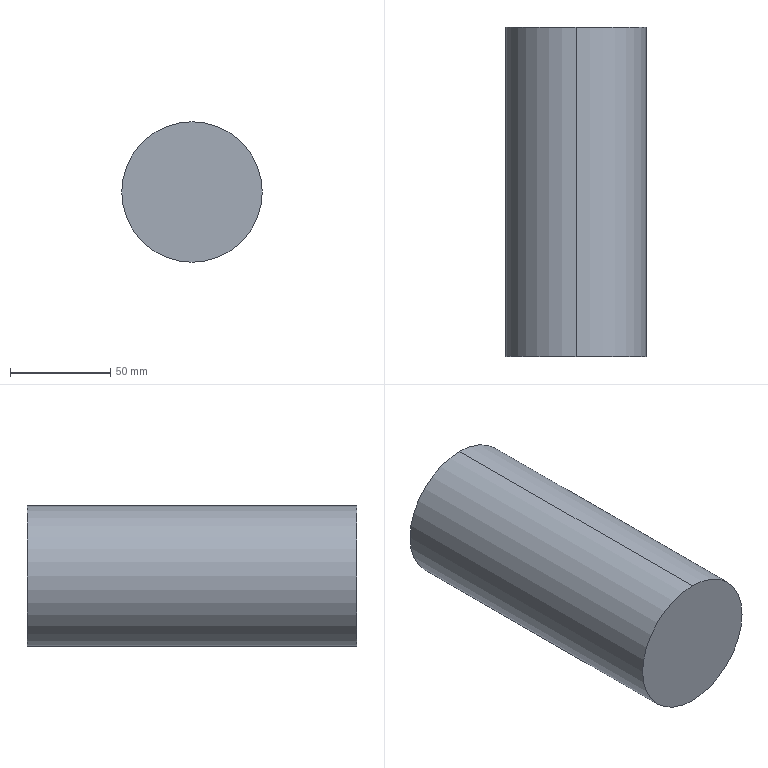Part | SolidWorks | features Extrusion 1 | 1 solid | 4 faces | box 70 x 163.9 x 70 mm | volume 630761 mm3 | cylinder 2 | plane 2 | commonest cylinder face diameters 70 x2
STEP:
#1=CARTESIAN_POINT('',(0.,163.9,35.));
#2=VERTEX_POINT('',#1);
#3=CARTESIAN_POINT('',(0.,163.9,-35.));
#4=VERTEX_POINT('',#3);
#5=CARTESIAN_POINT('',(0.,163.9,0.));
#6=DIRECTION('',(0.,1.,0.));
#7=DIRECTION('',(0.,0.,1.));
#8=AXIS2_PLACEMENT_3D('',#5,#6,#7);
#9=CIRCLE('',#8,35.);
#10=EDGE_CURVE('',#2,#4,#9,.T.);
#11=ORIENTED_EDGE('',*,*,#10,.F.);
#12=CARTESIAN_POINT('',(0.,0.,35.));
#13=VERTEX_POINT('',#12);
#14=CARTESIAN_POINT('',(0.,163.9,35.));
#15=DIRECTION('',(0.,-1.,0.));
#16=VECTOR('',#15,1000.);
#17=LINE('',#14,#16);
#18=EDGE_CURVE('',#2,#13,#17,.T.);
#19=ORIENTED_EDGE('',*,*,#18,.T.);
#20=CARTESIAN_POINT('',(0.,0.,-35.));
#21=VERTEX_POINT('',#20);
#22=CARTESIAN_POINT('',(0.,0.,0.));
#23=DIRECTION('',(0.,1.,0.));
#24=DIRECTION('',(0.,0.,1.));
#25=AXIS2_PLACEMENT_3D('',#22,#23,#24);
#26=CIRCLE('',#25,35.);
#27=EDGE_CURVE('',#13,#21,#26,.T.);
#28=ORIENTED_EDGE('',*,*,#27,.T.);
#29=CARTESIAN_POINT('',(0.,163.9,-35.));
#30=DIRECTION('',(0.,-1.,0.));
#31=VECTOR('',#30,1000.);
#32=LINE('',#29,#31);
#33=EDGE_CURVE('',#4,#21,#32,.T.);
#34=ORIENTED_EDGE('',*,*,#33,.F.);
#35=EDGE_LOOP('',(#11,#19,#28,#34));
#36=FACE_OUTER_BOUND('',#35,.T.);
#37=CARTESIAN_POINT('',(0.,163.9,0.));
#38=DIRECTION('',(0.,-1.,0.));
#39=DIRECTION('',(0.,0.,-1.));
#40=AXIS2_PLACEMENT_3D('',#37,#38,#39);
#41=CYLINDRICAL_SURFACE('',#40,35.);
#42=ADVANCED_FACE('',(#36),#41,.T.);
#43=ORIENTED_EDGE('',*,*,#18,.F.);
#44=CARTESIAN_POINT('',(0.,163.9,0.));
#45=DIRECTION('',(0.,1.,0.));
#46=DIRECTION('',(0.,0.,1.));
#47=AXIS2_PLACEMENT_3D('',#44,#45,#46);
#48=CIRCLE('',#47,35.);
#49=EDGE_CURVE('',#4,#2,#48,.T.);
#50=ORIENTED_EDGE('',*,*,#49,.F.);
#51=ORIENTED_EDGE('',*,*,#33,.T.);
#52=CARTESIAN_POINT('',(0.,0.,0.));
#53=DIRECTION('',(0.,1.,0.));
#54=DIRECTION('',(0.,0.,1.));
#55=AXIS2_PLACEMENT_3D('',#52,#53,#54);
#56=CIRCLE('',#55,35.);
#57=EDGE_CURVE('',#21,#13,#56,.T.);
#58=ORIENTED_EDGE('',*,*,#57,.T.);
#59=EDGE_LOOP('',(#43,#50,#51,#58));
#60=FACE_OUTER_BOUND('',#59,.T.);
#61=CARTESIAN_POINT('',(0.,163.9,0.));
#62=DIRECTION('',(0.,-1.,0.));
#63=DIRECTION('',(0.,0.,-1.));
#64=AXIS2_PLACEMENT_3D('',#61,#62,#63);
#65=CYLINDRICAL_SURFACE('',#64,35.);
#66=ADVANCED_FACE('',(#60),#65,.T.);
#67=ORIENTED_EDGE('',*,*,#49,.T.);
#68=ORIENTED_EDGE('',*,*,#10,.T.);
#69=EDGE_LOOP('',(#67,#68));
#70=FACE_OUTER_BOUND('',#69,.T.);
#71=CARTESIAN_POINT('',(0.,163.9,0.));
#72=DIRECTION('',(0.,1.,0.));
#73=DIRECTION('',(0.,0.,1.));
#74=AXIS2_PLACEMENT_3D('',#71,#72,#73);
#75=PLANE('',#74);
#76=ADVANCED_FACE('',(#70),#75,.T.);
#77=ORIENTED_EDGE('',*,*,#57,.F.);
#78=ORIENTED_EDGE('',*,*,#27,.F.);
#79=EDGE_LOOP('',(#77,#78));
#80=FACE_OUTER_BOUND('',#79,.T.);
#81=CARTESIAN_POINT('',(0.,0.,0.));
#82=DIRECTION('',(0.,1.,0.));
#83=DIRECTION('',(0.,0.,1.));
#84=AXIS2_PLACEMENT_3D('',#81,#82,#83);
#85=PLANE('',#84);
#86=ADVANCED_FACE('',(#80),#85,.F.);
#87=CLOSED_SHELL('',(#42,#66,#76,#86));
#88=MANIFOLD_SOLID_BREP('',#87);
#89=CARTESIAN_POINT('',(0.,0.,0.));
#90=DIRECTION('',(0.,0.,1.));
#91=DIRECTION('',(1.,0.,0.));
#92=AXIS2_PLACEMENT_3D('',#89,#90,#91);
#93=(LENGTH_UNIT()NAMED_UNIT(*)SI_UNIT(.MILLI.,.METRE.));
#94=UNCERTAINTY_MEASURE_WITH_UNIT(LENGTH_MEASURE(0.00001),#93,'','');
#95=(NAMED_UNIT(*)PLANE_ANGLE_UNIT()SI_UNIT($,.RADIAN.));
#96=(NAMED_UNIT(*)SI_UNIT($,.STERADIAN.)SOLID_ANGLE_UNIT());
#97=(GEOMETRIC_REPRESENTATION_CONTEXT(3)GLOBAL_UNCERTAINTY_ASSIGNED_CONTEXT((#94))GLOBAL_UNIT_ASSIGNED_CONTEXT((#93,#95,#96))REPRESENTATION_CONTEXT('',''));
#98=ADVANCED_BREP_SHAPE_REPRESENTATION('',(#88,#92),#97);